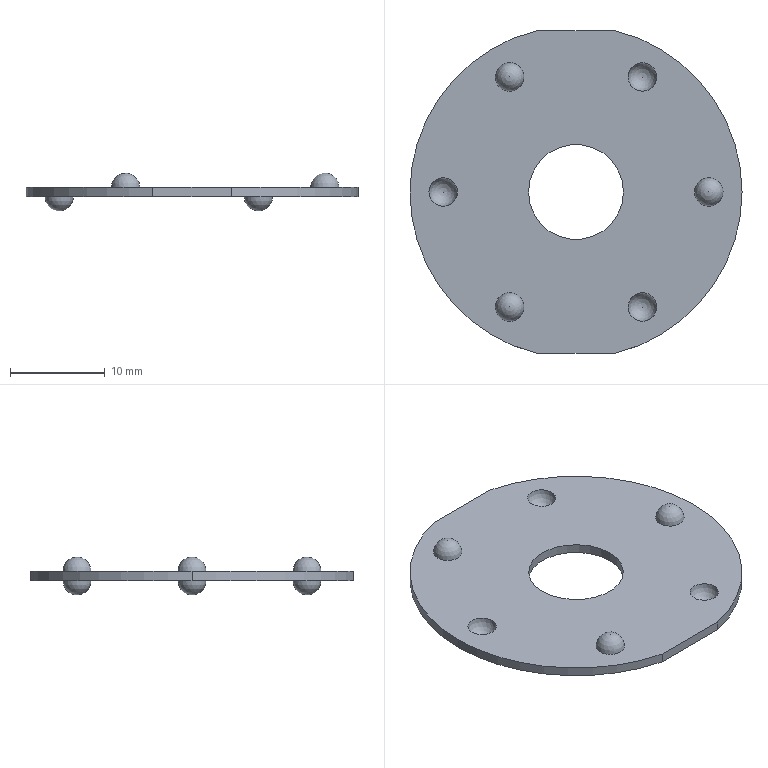Part | SolidWorks | features CirPattern 4, RevCut 2, Revolution 2, Extrusion 1, ICE 1 | 1 solid | 21 faces | box 35 x 34 x 4 mm | volume 890.444 mm3 | sphere 12 | cylinder 5 | plane 4 | commonest cylinder face diameters 35 x3 10 x2
STEP:
#1=CARTESIAN_POINT('',(-5.,0.,0.5));
#2=VERTEX_POINT('',#1);
#3=CARTESIAN_POINT('',(5.,0.,0.5));
#4=VERTEX_POINT('',#3);
#5=CARTESIAN_POINT('',(0.,0.,0.5));
#6=DIRECTION('',(0.,0.,1.));
#7=DIRECTION('',(1.,0.,0.));
#8=AXIS2_PLACEMENT_3D('',#5,#6,#7);
#9=CIRCLE('',#8,5.);
#10=EDGE_CURVE('',#2,#4,#9,.T.);
#11=ORIENTED_EDGE('',*,*,#10,.T.);
#12=CARTESIAN_POINT('',(5.,0.,-0.5));
#13=VERTEX_POINT('',#12);
#14=CARTESIAN_POINT('',(5.,0.,0.5));
#15=DIRECTION('',(0.,0.,-1.));
#16=VECTOR('',#15,1000.);
#17=LINE('',#14,#16);
#18=EDGE_CURVE('',#4,#13,#17,.T.);
#19=ORIENTED_EDGE('',*,*,#18,.T.);
#20=CARTESIAN_POINT('',(-5.,0.,-0.5));
#21=VERTEX_POINT('',#20);
#22=CARTESIAN_POINT('',(0.,0.,-0.5));
#23=DIRECTION('',(0.,0.,1.));
#24=DIRECTION('',(1.,0.,0.));
#25=AXIS2_PLACEMENT_3D('',#22,#23,#24);
#26=CIRCLE('',#25,5.);
#27=EDGE_CURVE('',#21,#13,#26,.T.);
#28=ORIENTED_EDGE('',*,*,#27,.F.);
#29=CARTESIAN_POINT('',(-5.,0.,0.5));
#30=DIRECTION('',(0.,0.,-1.));
#31=VECTOR('',#30,1000.);
#32=LINE('',#29,#31);
#33=EDGE_CURVE('',#2,#21,#32,.T.);
#34=ORIENTED_EDGE('',*,*,#33,.F.);
#35=EDGE_LOOP('',(#11,#19,#28,#34));
#36=FACE_OUTER_BOUND('',#35,.T.);
#37=CARTESIAN_POINT('',(0.,0.,0.5));
#38=DIRECTION('',(0.,0.,-1.));
#39=DIRECTION('',(-1.,0.,0.));
#40=AXIS2_PLACEMENT_3D('',#37,#38,#39);
#41=CYLINDRICAL_SURFACE('',#40,5.);
#42=ADVANCED_FACE('',(#36),#41,.F.);
#43=CARTESIAN_POINT('',(-17.5,0.,0.5));
#44=VERTEX_POINT('',#43);
#45=CARTESIAN_POINT('',(-4.153,-17.,0.5));
#46=VERTEX_POINT('',#45);
#47=CARTESIAN_POINT('',(0.,0.,0.5));
#48=DIRECTION('',(0.,0.,1.));
#49=DIRECTION('',(1.,0.,0.));
#50=AXIS2_PLACEMENT_3D('',#47,#48,#49);
#51=CIRCLE('',#50,17.5);
#52=EDGE_CURVE('',#44,#46,#51,.T.);
#53=ORIENTED_EDGE('',*,*,#52,.F.);
#54=CARTESIAN_POINT('',(-17.5,0.,-0.5));
#55=VERTEX_POINT('',#54);
#56=CARTESIAN_POINT('',(-17.5,0.,0.5));
#57=DIRECTION('',(0.,0.,-1.));
#58=VECTOR('',#57,1000.);
#59=LINE('',#56,#58);
#60=EDGE_CURVE('',#44,#55,#59,.T.);
#61=ORIENTED_EDGE('',*,*,#60,.T.);
#62=CARTESIAN_POINT('',(-4.153,-17.,-0.5));
#63=VERTEX_POINT('',#62);
#64=CARTESIAN_POINT('',(0.,0.,-0.5));
#65=DIRECTION('',(0.,0.,1.));
#66=DIRECTION('',(1.,0.,0.));
#67=AXIS2_PLACEMENT_3D('',#64,#65,#66);
#68=CIRCLE('',#67,17.5);
#69=EDGE_CURVE('',#55,#63,#68,.T.);
#70=ORIENTED_EDGE('',*,*,#69,.T.);
#71=CARTESIAN_POINT('',(-4.153,-17.,0.5));
#72=DIRECTION('',(0.,0.,1.));
#73=VECTOR('',#72,1000.);
#74=LINE('',#71,#73);
#75=EDGE_CURVE('',#63,#46,#74,.T.);
#76=ORIENTED_EDGE('',*,*,#75,.T.);
#77=EDGE_LOOP('',(#53,#61,#70,#76));
#78=FACE_OUTER_BOUND('',#77,.T.);
#79=CARTESIAN_POINT('',(0.,0.,0.5));
#80=DIRECTION('',(0.,0.,-1.));
#81=DIRECTION('',(-1.,0.,0.));
#82=AXIS2_PLACEMENT_3D('',#79,#80,#81);
#83=CYLINDRICAL_SURFACE('',#82,17.5);
#84=ADVANCED_FACE('',(#78),#83,.T.);
#85=ORIENTED_EDGE('',*,*,#60,.F.);
#86=CARTESIAN_POINT('',(-4.153,17.,0.5));
#87=VERTEX_POINT('',#86);
#88=CARTESIAN_POINT('',(0.,0.,0.5));
#89=DIRECTION('',(0.,0.,1.));
#90=DIRECTION('',(1.,0.,0.));
#91=AXIS2_PLACEMENT_3D('',#88,#89,#90);
#92=CIRCLE('',#91,17.5);
#93=EDGE_CURVE('',#87,#44,#92,.T.);
#94=ORIENTED_EDGE('',*,*,#93,.F.);
#95=CARTESIAN_POINT('',(-4.153,17.,-0.5));
#96=VERTEX_POINT('',#95);
#97=CARTESIAN_POINT('',(-4.153,17.,0.5));
#98=DIRECTION('',(0.,0.,-1.));
#99=VECTOR('',#98,1000.);
#100=LINE('',#97,#99);
#101=EDGE_CURVE('',#87,#96,#100,.T.);
#102=ORIENTED_EDGE('',*,*,#101,.T.);
#103=CARTESIAN_POINT('',(0.,0.,-0.5));
#104=DIRECTION('',(0.,0.,1.));
#105=DIRECTION('',(1.,0.,0.));
#106=AXIS2_PLACEMENT_3D('',#103,#104,#105);
#107=CIRCLE('',#106,17.5);
#108=EDGE_CURVE('',#96,#55,#107,.T.);
#109=ORIENTED_EDGE('',*,*,#108,.T.);
#110=EDGE_LOOP('',(#85,#94,#102,#109));
#111=FACE_OUTER_BOUND('',#110,.T.);
#112=CARTESIAN_POINT('',(0.,0.,0.5));
#113=DIRECTION('',(0.,0.,-1.));
#114=DIRECTION('',(-1.,0.,0.));
#115=AXIS2_PLACEMENT_3D('',#112,#113,#114);
#116=CYLINDRICAL_SURFACE('',#115,17.5);
#117=ADVANCED_FACE('',(#111),#116,.T.);
#118=CARTESIAN_POINT('',(8.5,12.124,0.5));
#119=VERTEX_POINT('',#118);
#120=CARTESIAN_POINT('',(5.5,12.124,0.5));
#121=VERTEX_POINT('',#120);
#122=CARTESIAN_POINT('',(7.,12.124,0.5));
#123=DIRECTION('',(0.,0.,1.));
#124=DIRECTION('',(1.,0.,0.));
#125=AXIS2_PLACEMENT_3D('',#122,#123,#124);
#126=CIRCLE('',#125,1.5);
#127=EDGE_CURVE('',#119,#121,#126,.T.);
#128=ORIENTED_EDGE('',*,*,#127,.F.);
#129=CARTESIAN_POINT('',(7.,12.124,0.5));
#130=DIRECTION('',(0.,0.,1.));
#131=DIRECTION('',(1.,0.,0.));
#132=AXIS2_PLACEMENT_3D('',#129,#130,#131);
#133=CIRCLE('',#132,1.5);
#134=EDGE_CURVE('',#121,#119,#133,.T.);
#135=ORIENTED_EDGE('',*,*,#134,.F.);
#136=EDGE_LOOP('',(#128,#135));
#137=FACE_BOUND('',#136,.T.);
#138=CARTESIAN_POINT('',(8.5,-12.124,0.5));
#139=VERTEX_POINT('',#138);
#140=CARTESIAN_POINT('',(5.5,-12.124,0.5));
#141=VERTEX_POINT('',#140);
#142=CARTESIAN_POINT('',(7.,-12.124,0.5));
#143=DIRECTION('',(0.,0.,1.));
#144=DIRECTION('',(1.,0.,0.));
#145=AXIS2_PLACEMENT_3D('',#142,#143,#144);
#146=CIRCLE('',#145,1.5);
#147=EDGE_CURVE('',#139,#141,#146,.T.);
#148=ORIENTED_EDGE('',*,*,#147,.F.);
#149=CARTESIAN_POINT('',(7.,-12.124,0.5));
#150=DIRECTION('',(0.,0.,1.));
#151=DIRECTION('',(1.,0.,0.));
#152=AXIS2_PLACEMENT_3D('',#149,#150,#151);
#153=CIRCLE('',#152,1.5);
#154=EDGE_CURVE('',#141,#139,#153,.T.);
#155=ORIENTED_EDGE('',*,*,#154,.F.);
#156=EDGE_LOOP('',(#148,#155));
#157=FACE_BOUND('',#156,.T.);
#158=CARTESIAN_POINT('',(-12.5,0.,0.5));
#159=VERTEX_POINT('',#158);
#160=CARTESIAN_POINT('',(-15.5,0.,0.5));
#161=VERTEX_POINT('',#160);
#162=CARTESIAN_POINT('',(-14.,0.,0.5));
#163=DIRECTION('',(0.,0.,1.));
#164=DIRECTION('',(1.,0.,0.));
#165=AXIS2_PLACEMENT_3D('',#162,#163,#164);
#166=CIRCLE('',#165,1.5);
#167=EDGE_CURVE('',#159,#161,#166,.T.);
#168=ORIENTED_EDGE('',*,*,#167,.F.);
#169=CARTESIAN_POINT('',(-14.,0.,0.5));
#170=DIRECTION('',(0.,0.,1.));
#171=DIRECTION('',(1.,0.,0.));
#172=AXIS2_PLACEMENT_3D('',#169,#170,#171);
#173=CIRCLE('',#172,1.5);
#174=EDGE_CURVE('',#161,#159,#173,.T.);
#175=ORIENTED_EDGE('',*,*,#174,.F.);
#176=EDGE_LOOP('',(#168,#175));
#177=FACE_BOUND('',#176,.T.);
#178=CARTESIAN_POINT('',(-5.5,-12.124,0.5));
#179=VERTEX_POINT('',#178);
#180=CARTESIAN_POINT('',(-8.5,-12.124,0.5));
#181=VERTEX_POINT('',#180);
#182=CARTESIAN_POINT('',(-7.,-12.124,0.5));
#183=DIRECTION('',(0.,0.,-1.));
#184=DIRECTION('',(1.,0.,0.));
#185=AXIS2_PLACEMENT_3D('',#182,#183,#184);
#186=CIRCLE('',#185,1.5);
#187=EDGE_CURVE('',#179,#181,#186,.T.);
#188=ORIENTED_EDGE('',*,*,#187,.T.);
#189=CARTESIAN_POINT('',(-7.,-12.124,0.5));
#190=DIRECTION('',(0.,0.,-1.));
#191=DIRECTION('',(1.,0.,0.));
#192=AXIS2_PLACEMENT_3D('',#189,#190,#191);
#193=CIRCLE('',#192,1.5);
#194=EDGE_CURVE('',#181,#179,#193,.T.);
#195=ORIENTED_EDGE('',*,*,#194,.T.);
#196=EDGE_LOOP('',(#188,#195));
#197=FACE_BOUND('',#196,.T.);
#198=CARTESIAN_POINT('',(-5.5,12.124,0.5));
#199=VERTEX_POINT('',#198);
#200=CARTESIAN_POINT('',(-8.5,12.124,0.5));
#201=VERTEX_POINT('',#200);
#202=CARTESIAN_POINT('',(-7.,12.124,0.5));
#203=DIRECTION('',(0.,0.,-1.));
#204=DIRECTION('',(1.,0.,0.));
#205=AXIS2_PLACEMENT_3D('',#202,#203,#204);
#206=CIRCLE('',#205,1.5);
#207=EDGE_CURVE('',#199,#201,#206,.T.);
#208=ORIENTED_EDGE('',*,*,#207,.T.);
#209=CARTESIAN_POINT('',(-7.,12.124,0.5));
#210=DIRECTION('',(0.,0.,-1.));
#211=DIRECTION('',(1.,0.,0.));
#212=AXIS2_PLACEMENT_3D('',#209,#210,#211);
#213=CIRCLE('',#212,1.5);
#214=EDGE_CURVE('',#201,#199,#213,.T.);
#215=ORIENTED_EDGE('',*,*,#214,.T.);
#216=EDGE_LOOP('',(#208,#215));
#217=FACE_BOUND('',#216,.T.);
#218=CARTESIAN_POINT('',(15.5,0.,0.5));
#219=VERTEX_POINT('',#218);
#220=CARTESIAN_POINT('',(12.5,0.,0.5));
#221=VERTEX_POINT('',#220);
#222=CARTESIAN_POINT('',(14.,0.,0.5));
#223=DIRECTION('',(0.,0.,-1.));
#224=DIRECTION('',(1.,0.,0.));
#225=AXIS2_PLACEMENT_3D('',#222,#223,#224);
#226=CIRCLE('',#225,1.5);
#227=EDGE_CURVE('',#219,#221,#226,.T.);
#228=ORIENTED_EDGE('',*,*,#227,.T.);
#229=CARTESIAN_POINT('',(14.,0.,0.5));
#230=DIRECTION('',(0.,0.,-1.));
#231=DIRECTION('',(1.,0.,0.));
#232=AXIS2_PLACEMENT_3D('',#229,#230,#231);
#233=CIRCLE('',#232,1.5);
#234=EDGE_CURVE('',#221,#219,#233,.T.);
#235=ORIENTED_EDGE('',*,*,#234,.T.);
#236=EDGE_LOOP('',(#228,#235));
#237=FACE_BOUND('',#236,.T.);
#238=CARTESIAN_POINT('',(4.153,17.,0.5));
#239=VERTEX_POINT('',#238);
#240=CARTESIAN_POINT('',(-12.615,17.,0.5));
#241=DIRECTION('',(1.,0.,0.));
#242=VECTOR('',#241,1000.);
#243=LINE('',#240,#242);
#244=EDGE_CURVE('',#87,#239,#243,.T.);
#245=ORIENTED_EDGE('',*,*,#244,.F.);
#246=ORIENTED_EDGE('',*,*,#93,.T.);
#247=ORIENTED_EDGE('',*,*,#52,.T.);
#248=CARTESIAN_POINT('',(4.153,-17.,0.5));
#249=VERTEX_POINT('',#248);
#250=CARTESIAN_POINT('',(-12.615,-17.,0.5));
#251=DIRECTION('',(-1.,0.,0.));
#252=VECTOR('',#251,1000.);
#253=LINE('',#250,#252);
#254=EDGE_CURVE('',#249,#46,#253,.T.);
#255=ORIENTED_EDGE('',*,*,#254,.F.);
#256=CARTESIAN_POINT('',(0.,0.,0.5));
#257=DIRECTION('',(0.,0.,1.));
#258=DIRECTION('',(1.,0.,0.));
#259=AXIS2_PLACEMENT_3D('',#256,#257,#258);
#260=CIRCLE('',#259,17.5);
#261=EDGE_CURVE('',#249,#239,#260,.T.);
#262=ORIENTED_EDGE('',*,*,#261,.T.);
#263=EDGE_LOOP('',(#245,#246,#247,#255,#262));
#264=FACE_OUTER_BOUND('',#263,.T.);
#265=ORIENTED_EDGE('',*,*,#10,.F.);
#266=CARTESIAN_POINT('',(0.,0.,0.5));
#267=DIRECTION('',(0.,0.,1.));
#268=DIRECTION('',(1.,0.,0.));
#269=AXIS2_PLACEMENT_3D('',#266,#267,#268);
#270=CIRCLE('',#269,5.);
#271=EDGE_CURVE('',#4,#2,#270,.T.);
#272=ORIENTED_EDGE('',*,*,#271,.F.);
#273=EDGE_LOOP('',(#265,#272));
#274=FACE_BOUND('',#273,.T.);
#275=CARTESIAN_POINT('',(0.,0.,0.5));
#276=DIRECTION('',(0.,0.,1.));
#277=DIRECTION('',(1.,0.,0.));
#278=AXIS2_PLACEMENT_3D('',#275,#276,#277);
#279=PLANE('',#278);
#280=ADVANCED_FACE('',(#137,#157,#177,#197,#217,#237,#264,#274),#279,.T.);
#281=CARTESIAN_POINT('',(8.5,12.124,-0.5));
#282=VERTEX_POINT('',#281);
#283=CARTESIAN_POINT('',(5.5,12.124,-0.5));
#284=VERTEX_POINT('',#283);
#285=CARTESIAN_POINT('',(7.,12.124,-0.5));
#286=DIRECTION('',(0.,0.,1.));
#287=DIRECTION('',(1.,0.,0.));
#288=AXIS2_PLACEMENT_3D('',#285,#286,#287);
#289=CIRCLE('',#288,1.5);
#290=EDGE_CURVE('',#282,#284,#289,.T.);
#291=ORIENTED_EDGE('',*,*,#290,.T.);
#292=CARTESIAN_POINT('',(7.,12.124,-0.5));
#293=DIRECTION('',(0.,0.,1.));
#294=DIRECTION('',(1.,0.,0.));
#295=AXIS2_PLACEMENT_3D('',#292,#293,#294);
#296=CIRCLE('',#295,1.5);
#297=EDGE_CURVE('',#284,#282,#296,.T.);
#298=ORIENTED_EDGE('',*,*,#297,.T.);
#299=EDGE_LOOP('',(#291,#298));
#300=FACE_BOUND('',#299,.T.);
#301=CARTESIAN_POINT('',(8.5,-12.124,-0.5));
#302=VERTEX_POINT('',#301);
#303=CARTESIAN_POINT('',(5.5,-12.124,-0.5));
#304=VERTEX_POINT('',#303);
#305=CARTESIAN_POINT('',(7.,-12.124,-0.5));
#306=DIRECTION('',(0.,0.,1.));
#307=DIRECTION('',(1.,0.,0.));
#308=AXIS2_PLACEMENT_3D('',#305,#306,#307);
#309=CIRCLE('',#308,1.5);
#310=EDGE_CURVE('',#302,#304,#309,.T.);
#311=ORIENTED_EDGE('',*,*,#310,.T.);
#312=CARTESIAN_POINT('',(7.,-12.124,-0.5));
#313=DIRECTION('',(0.,0.,1.));
#314=DIRECTION('',(1.,0.,0.));
#315=AXIS2_PLACEMENT_3D('',#312,#313,#314);
#316=CIRCLE('',#315,1.5);
#317=EDGE_CURVE('',#304,#302,#316,.T.);
#318=ORIENTED_EDGE('',*,*,#317,.T.);
#319=EDGE_LOOP('',(#311,#318));
#320=FACE_BOUND('',#319,.T.);
#321=CARTESIAN_POINT('',(-12.5,0.,-0.5));
#322=VERTEX_POINT('',#321);
#323=CARTESIAN_POINT('',(-15.5,0.,-0.5));
#324=VERTEX_POINT('',#323);
#325=CARTESIAN_POINT('',(-14.,0.,-0.5));
#326=DIRECTION('',(0.,0.,1.));
#327=DIRECTION('',(1.,0.,0.));
#328=AXIS2_PLACEMENT_3D('',#325,#326,#327);
#329=CIRCLE('',#328,1.5);
#330=EDGE_CURVE('',#322,#324,#329,.T.);
#331=ORIENTED_EDGE('',*,*,#330,.T.);
#332=CARTESIAN_POINT('',(-14.,0.,-0.5));
#333=DIRECTION('',(0.,0.,1.));
#334=DIRECTION('',(1.,0.,0.));
#335=AXIS2_PLACEMENT_3D('',#332,#333,#334);
#336=CIRCLE('',#335,1.5);
#337=EDGE_CURVE('',#324,#322,#336,.T.);
#338=ORIENTED_EDGE('',*,*,#337,.T.);
#339=EDGE_LOOP('',(#331,#338));
#340=FACE_BOUND('',#339,.T.);
#341=CARTESIAN_POINT('',(-8.118,-12.124,-0.5));
#342=VERTEX_POINT('',#341);
#343=CARTESIAN_POINT('',(-5.882,-12.124,-0.5));
#344=VERTEX_POINT('',#343);
#345=CARTESIAN_POINT('',(-7.,-12.124,-0.5));
#346=DIRECTION('',(0.,0.,-1.));
#347=DIRECTION('',(-1.,0.,0.));
#348=AXIS2_PLACEMENT_3D('',#345,#346,#347);
#349=CIRCLE('',#348,1.118);
#350=EDGE_CURVE('',#342,#344,#349,.T.);
#351=ORIENTED_EDGE('',*,*,#350,.F.);
#352=CARTESIAN_POINT('',(-7.,-12.124,-0.5));
#353=DIRECTION('',(0.,0.,-1.));
#354=DIRECTION('',(-1.,0.,0.));
#355=AXIS2_PLACEMENT_3D('',#352,#353,#354);
#356=CIRCLE('',#355,1.118);
#357=EDGE_CURVE('',#344,#342,#356,.T.);
#358=ORIENTED_EDGE('',*,*,#357,.F.);
#359=EDGE_LOOP('',(#351,#358));
#360=FACE_BOUND('',#359,.T.);
#361=CARTESIAN_POINT('',(-8.118,12.124,-0.5));
#362=VERTEX_POINT('',#361);
#363=CARTESIAN_POINT('',(-5.882,12.124,-0.5));
#364=VERTEX_POINT('',#363);
#365=CARTESIAN_POINT('',(-7.,12.124,-0.5));
#366=DIRECTION('',(0.,0.,-1.));
#367=DIRECTION('',(-1.,0.,0.));
#368=AXIS2_PLACEMENT_3D('',#365,#366,#367);
#369=CIRCLE('',#368,1.118);
#370=EDGE_CURVE('',#362,#364,#369,.T.);
#371=ORIENTED_EDGE('',*,*,#370,.F.);
#372=CARTESIAN_POINT('',(-7.,12.124,-0.5));
#373=DIRECTION('',(0.,0.,-1.));
#374=DIRECTION('',(-1.,0.,0.));
#375=AXIS2_PLACEMENT_3D('',#372,#373,#374);
#376=CIRCLE('',#375,1.118);
#377=EDGE_CURVE('',#364,#362,#376,.T.);
#378=ORIENTED_EDGE('',*,*,#377,.F.);
#379=EDGE_LOOP('',(#371,#378));
#380=FACE_BOUND('',#379,.T.);
#381=CARTESIAN_POINT('',(12.882,0.,-0.5));
#382=VERTEX_POINT('',#381);
#383=CARTESIAN_POINT('',(15.118,0.,-0.5));
#384=VERTEX_POINT('',#383);
#385=CARTESIAN_POINT('',(14.,0.,-0.5));
#386=DIRECTION('',(0.,0.,-1.));
#387=DIRECTION('',(-1.,0.,0.));
#388=AXIS2_PLACEMENT_3D('',#385,#386,#387);
#389=CIRCLE('',#388,1.118);
#390=EDGE_CURVE('',#382,#384,#389,.T.);
#391=ORIENTED_EDGE('',*,*,#390,.F.);
#392=CARTESIAN_POINT('',(14.,0.,-0.5));
#393=DIRECTION('',(0.,0.,-1.));
#394=DIRECTION('',(-1.,0.,0.));
#395=AXIS2_PLACEMENT_3D('',#392,#393,#394);
#396=CIRCLE('',#395,1.118);
#397=EDGE_CURVE('',#384,#382,#396,.T.);
#398=ORIENTED_EDGE('',*,*,#397,.F.);
#399=EDGE_LOOP('',(#391,#398));
#400=FACE_BOUND('',#399,.T.);
#401=ORIENTED_EDGE('',*,*,#108,.F.);
#402=CARTESIAN_POINT('',(4.153,17.,-0.5));
#403=VERTEX_POINT('',#402);
#404=CARTESIAN_POINT('',(-12.615,17.,-0.5));
#405=DIRECTION('',(1.,0.,0.));
#406=VECTOR('',#405,1000.);
#407=LINE('',#404,#406);
#408=EDGE_CURVE('',#96,#403,#407,.T.);
#409=ORIENTED_EDGE('',*,*,#408,.T.);
#410=CARTESIAN_POINT('',(4.153,-17.,-0.5));
#411=VERTEX_POINT('',#410);
#412=CARTESIAN_POINT('',(0.,0.,-0.5));
#413=DIRECTION('',(0.,0.,1.));
#414=DIRECTION('',(1.,0.,0.));
#415=AXIS2_PLACEMENT_3D('',#412,#413,#414);
#416=CIRCLE('',#415,17.5);
#417=EDGE_CURVE('',#411,#403,#416,.T.);
#418=ORIENTED_EDGE('',*,*,#417,.F.);
#419=CARTESIAN_POINT('',(-12.615,-17.,-0.5));
#420=DIRECTION('',(-1.,0.,0.));
#421=VECTOR('',#420,1000.);
#422=LINE('',#419,#421);
#423=EDGE_CURVE('',#411,#63,#422,.T.);
#424=ORIENTED_EDGE('',*,*,#423,.T.);
#425=ORIENTED_EDGE('',*,*,#69,.F.);
#426=EDGE_LOOP('',(#401,#409,#418,#424,#425));
#427=FACE_OUTER_BOUND('',#426,.T.);
#428=ORIENTED_EDGE('',*,*,#27,.T.);
#429=CARTESIAN_POINT('',(0.,0.,-0.5));
#430=DIRECTION('',(0.,0.,1.));
#431=DIRECTION('',(1.,0.,0.));
#432=AXIS2_PLACEMENT_3D('',#429,#430,#431);
#433=CIRCLE('',#432,5.);
#434=EDGE_CURVE('',#13,#21,#433,.T.);
#435=ORIENTED_EDGE('',*,*,#434,.T.);
#436=EDGE_LOOP('',(#428,#435));
#437=FACE_BOUND('',#436,.T.);
#438=CARTESIAN_POINT('',(0.,0.,-0.5));
#439=DIRECTION('',(0.,0.,1.));
#440=DIRECTION('',(1.,0.,0.));
#441=AXIS2_PLACEMENT_3D('',#438,#439,#440);
#442=PLANE('',#441);
#443=ADVANCED_FACE('',(#300,#320,#340,#360,#380,#400,#427,#437),#442,.F.);
#444=ORIENTED_EDGE('',*,*,#417,.T.);
#445=CARTESIAN_POINT('',(4.153,17.,0.5));
#446=DIRECTION('',(0.,0.,1.));
#447=VECTOR('',#446,1000.);
#448=LINE('',#445,#447);
#449=EDGE_CURVE('',#403,#239,#448,.T.);
#450=ORIENTED_EDGE('',*,*,#449,.T.);
#451=ORIENTED_EDGE('',*,*,#261,.F.);
#452=CARTESIAN_POINT('',(4.153,-17.,0.5));
#453=DIRECTION('',(0.,0.,-1.));
#454=VECTOR('',#453,1000.);
#455=LINE('',#452,#454);
#456=EDGE_CURVE('',#249,#411,#455,.T.);
#457=ORIENTED_EDGE('',*,*,#456,.T.);
#458=EDGE_LOOP('',(#444,#450,#451,#457));
#459=FACE_OUTER_BOUND('',#458,.T.);
#460=CARTESIAN_POINT('',(0.,0.,0.5));
#461=DIRECTION('',(0.,0.,-1.));
#462=DIRECTION('',(-1.,0.,0.));
#463=AXIS2_PLACEMENT_3D('',#460,#461,#462);
#464=CYLINDRICAL_SURFACE('',#463,17.5);
#465=ADVANCED_FACE('',(#459),#464,.T.);
#466=ORIENTED_EDGE('',*,*,#18,.F.);
#467=ORIENTED_EDGE('',*,*,#271,.T.);
#468=ORIENTED_EDGE('',*,*,#33,.T.);
#469=ORIENTED_EDGE('',*,*,#434,.F.);
#470=EDGE_LOOP('',(#466,#467,#468,#469));
#471=FACE_OUTER_BOUND('',#470,.T.);
#472=CARTESIAN_POINT('',(0.,0.,0.5));
#473=DIRECTION('',(0.,0.,-1.));
#474=DIRECTION('',(-1.,0.,0.));
#475=AXIS2_PLACEMENT_3D('',#472,#473,#474);
#476=CYLINDRICAL_SURFACE('',#475,5.);
#477=ADVANCED_FACE('',(#471),#476,.F.);
#478=ORIENTED_EDGE('',*,*,#254,.T.);
#479=ORIENTED_EDGE('',*,*,#75,.F.);
#480=ORIENTED_EDGE('',*,*,#423,.F.);
#481=ORIENTED_EDGE('',*,*,#456,.F.);
#482=EDGE_LOOP('',(#478,#479,#480,#481));
#483=FACE_OUTER_BOUND('',#482,.T.);
#484=CARTESIAN_POINT('',(-12.615,-17.,-0.5));
#485=DIRECTION('',(0.,1.,0.));
#486=DIRECTION('',(0.,0.,1.));
#487=AXIS2_PLACEMENT_3D('',#484,#485,#486);
#488=PLANE('',#487);
#489=ADVANCED_FACE('',(#483),#488,.F.);
#490=ORIENTED_EDGE('',*,*,#244,.T.);
#491=ORIENTED_EDGE('',*,*,#449,.F.);
#492=ORIENTED_EDGE('',*,*,#408,.F.);
#493=ORIENTED_EDGE('',*,*,#101,.F.);
#494=EDGE_LOOP('',(#490,#491,#492,#493));
#495=FACE_OUTER_BOUND('',#494,.T.);
#496=CARTESIAN_POINT('',(-12.615,17.,-0.5));
#497=DIRECTION('',(0.,-1.,0.));
#498=DIRECTION('',(0.,0.,-1.));
#499=AXIS2_PLACEMENT_3D('',#496,#497,#498);
#500=PLANE('',#499);
#501=ADVANCED_FACE('',(#495),#500,.F.);
#502=ORIENTED_EDGE('',*,*,#227,.F.);
#503=ORIENTED_EDGE('',*,*,#234,.F.);
#504=EDGE_LOOP('',(#502,#503));
#505=FACE_OUTER_BOUND('',#504,.T.);
#506=CARTESIAN_POINT('',(14.,0.,0.5));
#507=DIRECTION('',(0.,0.,-1.));
#508=DIRECTION('',(1.,0.,0.));
#509=AXIS2_PLACEMENT_3D('',#506,#507,#508);
#510=SPHERICAL_SURFACE('',#509,1.5);
#511=ADVANCED_FACE('',(#505),#510,.T.);
#512=ORIENTED_EDGE('',*,*,#207,.F.);
#513=ORIENTED_EDGE('',*,*,#214,.F.);
#514=EDGE_LOOP('',(#512,#513));
#515=FACE_OUTER_BOUND('',#514,.T.);
#516=CARTESIAN_POINT('',(-7.,12.124,0.5));
#517=DIRECTION('',(0.,0.,-1.));
#518=DIRECTION('',(-0.5,0.866,0.));
#519=AXIS2_PLACEMENT_3D('',#516,#517,#518);
#520=SPHERICAL_SURFACE('',#519,1.5);
#521=ADVANCED_FACE('',(#515),#520,.T.);
#522=ORIENTED_EDGE('',*,*,#187,.F.);
#523=ORIENTED_EDGE('',*,*,#194,.F.);
#524=EDGE_LOOP('',(#522,#523));
#525=FACE_OUTER_BOUND('',#524,.T.);
#526=CARTESIAN_POINT('',(-7.,-12.124,0.5));
#527=DIRECTION('',(0.,0.,-1.));
#528=DIRECTION('',(-0.5,-0.866,0.));
#529=AXIS2_PLACEMENT_3D('',#526,#527,#528);
#530=SPHERICAL_SURFACE('',#529,1.5);
#531=ADVANCED_FACE('',(#525),#530,.T.);
#532=ORIENTED_EDGE('',*,*,#330,.F.);
#533=ORIENTED_EDGE('',*,*,#337,.F.);
#534=EDGE_LOOP('',(#532,#533));
#535=FACE_OUTER_BOUND('',#534,.T.);
#536=CARTESIAN_POINT('',(-14.,0.,-0.5));
#537=DIRECTION('',(0.,0.,1.));
#538=DIRECTION('',(1.,0.,0.));
#539=AXIS2_PLACEMENT_3D('',#536,#537,#538);
#540=SPHERICAL_SURFACE('',#539,1.5);
#541=ADVANCED_FACE('',(#535),#540,.T.);
#542=ORIENTED_EDGE('',*,*,#310,.F.);
#543=ORIENTED_EDGE('',*,*,#317,.F.);
#544=EDGE_LOOP('',(#542,#543));
#545=FACE_OUTER_BOUND('',#544,.T.);
#546=CARTESIAN_POINT('',(7.,-12.124,-0.5));
#547=DIRECTION('',(0.,0.,1.));
#548=DIRECTION('',(-0.5,0.866,0.));
#549=AXIS2_PLACEMENT_3D('',#546,#547,#548);
#550=SPHERICAL_SURFACE('',#549,1.5);
#551=ADVANCED_FACE('',(#545),#550,.T.);
#552=ORIENTED_EDGE('',*,*,#290,.F.);
#553=ORIENTED_EDGE('',*,*,#297,.F.);
#554=EDGE_LOOP('',(#552,#553));
#555=FACE_OUTER_BOUND('',#554,.T.);
#556=CARTESIAN_POINT('',(7.,12.124,-0.5));
#557=DIRECTION('',(0.,0.,1.));
#558=DIRECTION('',(-0.5,-0.866,0.));
#559=AXIS2_PLACEMENT_3D('',#556,#557,#558);
#560=SPHERICAL_SURFACE('',#559,1.5);
#561=ADVANCED_FACE('',(#555),#560,.T.);
#562=ORIENTED_EDGE('',*,*,#167,.T.);
#563=ORIENTED_EDGE('',*,*,#174,.T.);
#564=EDGE_LOOP('',(#562,#563));
#565=FACE_OUTER_BOUND('',#564,.T.);
#566=CARTESIAN_POINT('',(-14.,0.,0.5));
#567=DIRECTION('',(0.,0.,-1.));
#568=DIRECTION('',(1.,0.,0.));
#569=AXIS2_PLACEMENT_3D('',#566,#567,#568);
#570=SPHERICAL_SURFACE('',#569,1.5);
#571=ADVANCED_FACE('',(#565),#570,.F.);
#572=ORIENTED_EDGE('',*,*,#147,.T.);
#573=ORIENTED_EDGE('',*,*,#154,.T.);
#574=EDGE_LOOP('',(#572,#573));
#575=FACE_OUTER_BOUND('',#574,.T.);
#576=CARTESIAN_POINT('',(7.,-12.124,0.5));
#577=DIRECTION('',(0.,0.,-1.));
#578=DIRECTION('',(-0.5,0.866,0.));
#579=AXIS2_PLACEMENT_3D('',#576,#577,#578);
#580=SPHERICAL_SURFACE('',#579,1.5);
#581=ADVANCED_FACE('',(#575),#580,.F.);
#582=ORIENTED_EDGE('',*,*,#127,.T.);
#583=ORIENTED_EDGE('',*,*,#134,.T.);
#584=EDGE_LOOP('',(#582,#583));
#585=FACE_OUTER_BOUND('',#584,.T.);
#586=CARTESIAN_POINT('',(7.,12.124,0.5));
#587=DIRECTION('',(0.,0.,-1.));
#588=DIRECTION('',(-0.5,-0.866,0.));
#589=AXIS2_PLACEMENT_3D('',#586,#587,#588);
#590=SPHERICAL_SURFACE('',#589,1.5);
#591=ADVANCED_FACE('',(#585),#590,.F.);
#592=ORIENTED_EDGE('',*,*,#390,.T.);
#593=ORIENTED_EDGE('',*,*,#397,.T.);
#594=EDGE_LOOP('',(#592,#593));
#595=FACE_OUTER_BOUND('',#594,.T.);
#596=CARTESIAN_POINT('',(14.,0.,-0.5));
#597=DIRECTION('',(0.,0.,1.));
#598=DIRECTION('',(1.,0.,0.));
#599=AXIS2_PLACEMENT_3D('',#596,#597,#598);
#600=SPHERICAL_SURFACE('',#599,1.118);
#601=ADVANCED_FACE('',(#595),#600,.F.);
#602=ORIENTED_EDGE('',*,*,#370,.T.);
#603=ORIENTED_EDGE('',*,*,#377,.T.);
#604=EDGE_LOOP('',(#602,#603));
#605=FACE_OUTER_BOUND('',#604,.T.);
#606=CARTESIAN_POINT('',(-7.,12.124,-0.5));
#607=DIRECTION('',(0.,0.,1.));
#608=DIRECTION('',(-0.5,0.866,0.));
#609=AXIS2_PLACEMENT_3D('',#606,#607,#608);
#610=SPHERICAL_SURFACE('',#609,1.118);
#611=ADVANCED_FACE('',(#605),#610,.F.);
#612=ORIENTED_EDGE('',*,*,#350,.T.);
#613=ORIENTED_EDGE('',*,*,#357,.T.);
#614=EDGE_LOOP('',(#612,#613));
#615=FACE_OUTER_BOUND('',#614,.T.);
#616=CARTESIAN_POINT('',(-7.,-12.124,-0.5));
#617=DIRECTION('',(0.,0.,1.));
#618=DIRECTION('',(-0.5,-0.866,0.));
#619=AXIS2_PLACEMENT_3D('',#616,#617,#618);
#620=SPHERICAL_SURFACE('',#619,1.118);
#621=ADVANCED_FACE('',(#615),#620,.F.);
#622=CLOSED_SHELL('',(#42,#84,#117,#280,#443,#465,#477,#489,#501,#511,#521,#531,#541,#551,#561,#571,#581,#591,#601,#611,#621));
#623=MANIFOLD_SOLID_BREP('',#622);
#624=CARTESIAN_POINT('',(0.,0.,0.));
#625=DIRECTION('',(0.,0.,1.));
#626=DIRECTION('',(1.,0.,0.));
#627=AXIS2_PLACEMENT_3D('',#624,#625,#626);
#628=(LENGTH_UNIT()NAMED_UNIT(*)SI_UNIT(.MILLI.,.METRE.));
#629=UNCERTAINTY_MEASURE_WITH_UNIT(LENGTH_MEASURE(0.00001),#628,'','');
#630=(NAMED_UNIT(*)PLANE_ANGLE_UNIT()SI_UNIT($,.RADIAN.));
#631=(NAMED_UNIT(*)SI_UNIT($,.STERADIAN.)SOLID_ANGLE_UNIT());
#632=(GEOMETRIC_REPRESENTATION_CONTEXT(3)GLOBAL_UNCERTAINTY_ASSIGNED_CONTEXT((#629))GLOBAL_UNIT_ASSIGNED_CONTEXT((#628,#630,#631))REPRESENTATION_CONTEXT('',''));
#633=ADVANCED_BREP_SHAPE_REPRESENTATION('',(#623,#627),#632);